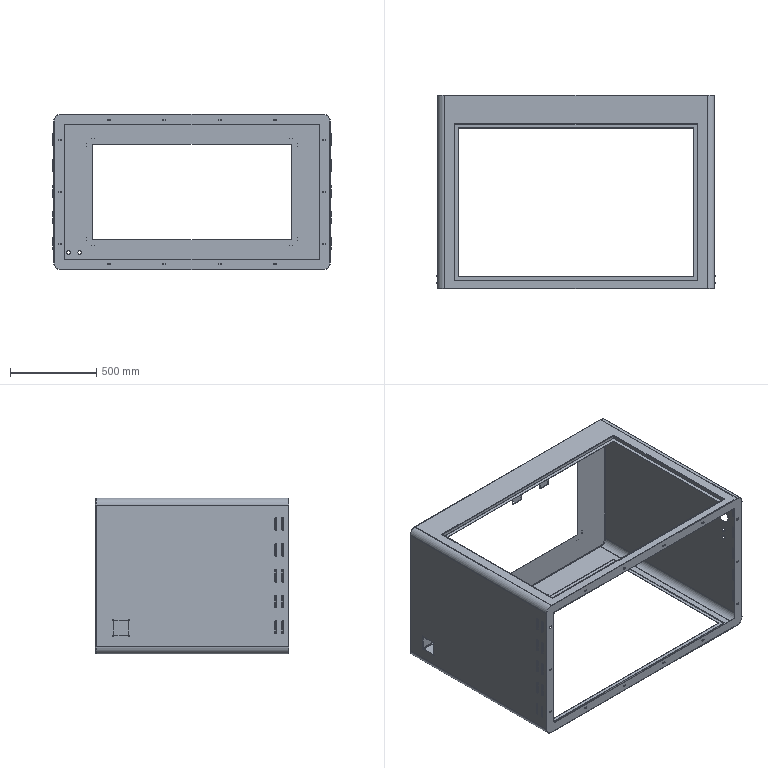Part | STEP file | b-005 | 1 solid | 566 faces | box 1610 x 1120 x 900 mm | volume 8822368 mm3 | cylinder 286 | plane 192 | sphere 80 | torus 8 | commonest cylinder face diameters 6 x88 10 x64 3.3 x40 8 x28 4.6 x24 4 x12